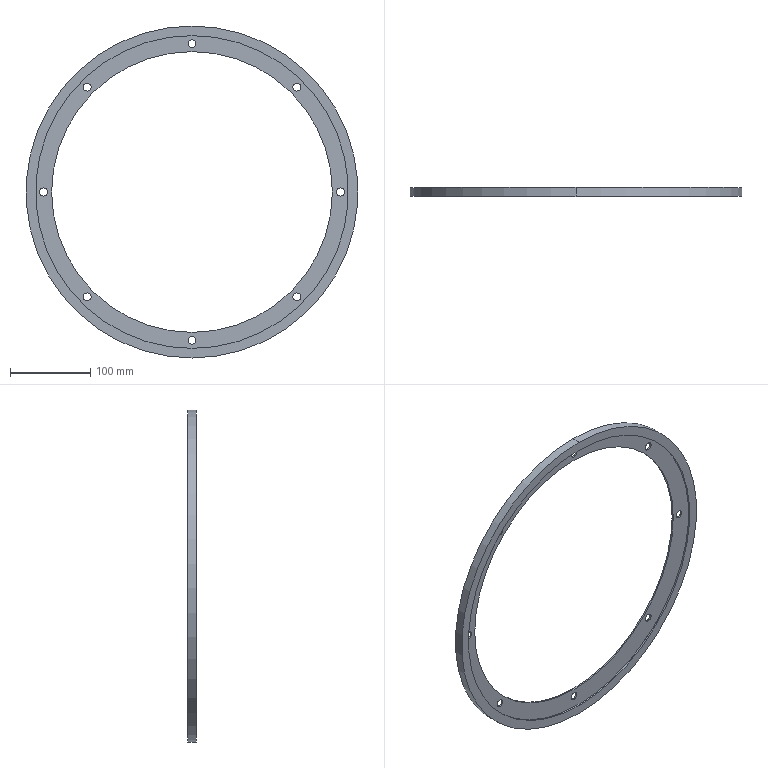Part | SolidWorks | features ICE 2, Extrusion 1 | 1 solid | 28 faces | box 414 x 11 x 414 mm | volume 123980 mm3 | cylinder 24 | plane 4 | commonest cylinder face diameters 10 x16 350 x2 390 x2 410 x2 414 x2
STEP:
#1=CARTESIAN_POINT('',(0.,-9.,195.));
#2=VERTEX_POINT('',#1);
#3=CARTESIAN_POINT('',(0.,-9.,-195.));
#4=VERTEX_POINT('',#3);
#5=CARTESIAN_POINT('',(0.,-9.,0.));
#6=DIRECTION('',(0.,-1.,0.));
#7=DIRECTION('',(0.,0.,-1.));
#8=AXIS2_PLACEMENT_3D('',#5,#6,#7);
#9=CIRCLE('',#8,195.);
#10=EDGE_CURVE('',#2,#4,#9,.T.);
#11=ORIENTED_EDGE('',*,*,#10,.T.);
#12=CARTESIAN_POINT('',(0.,-7.,-195.));
#13=VERTEX_POINT('',#12);
#14=CARTESIAN_POINT('',(0.,-9.,-195.));
#15=DIRECTION('',(0.,1.,0.));
#16=VECTOR('',#15,1000.);
#17=LINE('',#14,#16);
#18=EDGE_CURVE('',#4,#13,#17,.T.);
#19=ORIENTED_EDGE('',*,*,#18,.T.);
#20=CARTESIAN_POINT('',(0.,-7.,195.));
#21=VERTEX_POINT('',#20);
#22=CARTESIAN_POINT('',(0.,-7.,0.));
#23=DIRECTION('',(0.,-1.,0.));
#24=DIRECTION('',(0.,0.,-1.));
#25=AXIS2_PLACEMENT_3D('',#22,#23,#24);
#26=CIRCLE('',#25,195.);
#27=EDGE_CURVE('',#21,#13,#26,.T.);
#28=ORIENTED_EDGE('',*,*,#27,.F.);
#29=CARTESIAN_POINT('',(0.,-9.,195.));
#30=DIRECTION('',(0.,1.,0.));
#31=VECTOR('',#30,1000.);
#32=LINE('',#29,#31);
#33=EDGE_CURVE('',#2,#21,#32,.T.);
#34=ORIENTED_EDGE('',*,*,#33,.F.);
#35=EDGE_LOOP('',(#11,#19,#28,#34));
#36=FACE_OUTER_BOUND('',#35,.T.);
#37=CARTESIAN_POINT('',(0.,-9.,0.));
#38=DIRECTION('',(0.,1.,0.));
#39=DIRECTION('',(0.,0.,1.));
#40=AXIS2_PLACEMENT_3D('',#37,#38,#39);
#41=CYLINDRICAL_SURFACE('',#40,195.);
#42=ADVANCED_FACE('',(#36),#41,.F.);
#43=CARTESIAN_POINT('',(0.,2.,-207.));
#44=VERTEX_POINT('',#43);
#45=CARTESIAN_POINT('',(0.,2.,207.));
#46=VERTEX_POINT('',#45);
#47=CARTESIAN_POINT('',(0.,2.,0.));
#48=DIRECTION('',(0.,-1.,0.));
#49=DIRECTION('',(0.,0.,-1.));
#50=AXIS2_PLACEMENT_3D('',#47,#48,#49);
#51=CIRCLE('',#50,207.);
#52=EDGE_CURVE('',#44,#46,#51,.T.);
#53=ORIENTED_EDGE('',*,*,#52,.T.);
#54=CARTESIAN_POINT('',(0.,-9.,207.));
#55=VERTEX_POINT('',#54);
#56=CARTESIAN_POINT('',(0.,2.,207.));
#57=DIRECTION('',(0.,-1.,0.));
#58=VECTOR('',#57,1000.);
#59=LINE('',#56,#58);
#60=EDGE_CURVE('',#46,#55,#59,.T.);
#61=ORIENTED_EDGE('',*,*,#60,.T.);
#62=CARTESIAN_POINT('',(0.,-9.,-207.));
#63=VERTEX_POINT('',#62);
#64=CARTESIAN_POINT('',(0.,-9.,0.));
#65=DIRECTION('',(0.,-1.,0.));
#66=DIRECTION('',(0.,0.,-1.));
#67=AXIS2_PLACEMENT_3D('',#64,#65,#66);
#68=CIRCLE('',#67,207.);
#69=EDGE_CURVE('',#63,#55,#68,.T.);
#70=ORIENTED_EDGE('',*,*,#69,.F.);
#71=CARTESIAN_POINT('',(0.,2.,-207.));
#72=DIRECTION('',(0.,-1.,0.));
#73=VECTOR('',#72,1000.);
#74=LINE('',#71,#73);
#75=EDGE_CURVE('',#44,#63,#74,.T.);
#76=ORIENTED_EDGE('',*,*,#75,.F.);
#77=EDGE_LOOP('',(#53,#61,#70,#76));
#78=FACE_OUTER_BOUND('',#77,.T.);
#79=CARTESIAN_POINT('',(0.,2.,0.));
#80=DIRECTION('',(0.,-1.,0.));
#81=DIRECTION('',(0.,0.,-1.));
#82=AXIS2_PLACEMENT_3D('',#79,#80,#81);
#83=CYLINDRICAL_SURFACE('',#82,207.);
#84=ADVANCED_FACE('',(#78),#83,.T.);
#85=CARTESIAN_POINT('',(0.,0.,-205.));
#86=VERTEX_POINT('',#85);
#87=CARTESIAN_POINT('',(0.,0.,205.));
#88=VERTEX_POINT('',#87);
#89=CARTESIAN_POINT('',(0.,0.,0.));
#90=DIRECTION('',(0.,1.,0.));
#91=DIRECTION('',(0.,0.,1.));
#92=AXIS2_PLACEMENT_3D('',#89,#90,#91);
#93=CIRCLE('',#92,205.);
#94=EDGE_CURVE('',#86,#88,#93,.T.);
#95=ORIENTED_EDGE('',*,*,#94,.T.);
#96=CARTESIAN_POINT('',(0.,-7.,205.));
#97=VERTEX_POINT('',#96);
#98=CARTESIAN_POINT('',(0.,2.,205.));
#99=DIRECTION('',(0.,-1.,0.));
#100=VECTOR('',#99,1000.);
#101=LINE('',#98,#100);
#102=EDGE_CURVE('',#88,#97,#101,.T.);
#103=ORIENTED_EDGE('',*,*,#102,.T.);
#104=CARTESIAN_POINT('',(0.,-7.,-205.));
#105=VERTEX_POINT('',#104);
#106=CARTESIAN_POINT('',(0.,-7.,0.));
#107=DIRECTION('',(0.,-1.,0.));
#108=DIRECTION('',(0.,0.,-1.));
#109=AXIS2_PLACEMENT_3D('',#106,#107,#108);
#110=CIRCLE('',#109,205.);
#111=EDGE_CURVE('',#97,#105,#110,.T.);
#112=ORIENTED_EDGE('',*,*,#111,.T.);
#113=CARTESIAN_POINT('',(0.,2.,-205.));
#114=DIRECTION('',(0.,-1.,0.));
#115=VECTOR('',#114,1000.);
#116=LINE('',#113,#115);
#117=EDGE_CURVE('',#86,#105,#116,.T.);
#118=ORIENTED_EDGE('',*,*,#117,.F.);
#119=EDGE_LOOP('',(#95,#103,#112,#118));
#120=FACE_OUTER_BOUND('',#119,.T.);
#121=CARTESIAN_POINT('',(0.,2.,0.));
#122=DIRECTION('',(0.,-1.,0.));
#123=DIRECTION('',(0.,0.,-1.));
#124=AXIS2_PLACEMENT_3D('',#121,#122,#123);
#125=CYLINDRICAL_SURFACE('',#124,205.);
#126=ADVANCED_FACE('',(#120),#125,.F.);
#127=CARTESIAN_POINT('',(-130.815,2.,125.815));
#128=VERTEX_POINT('',#127);
#129=CARTESIAN_POINT('',(-130.815,2.,135.815));
#130=VERTEX_POINT('',#129);
#131=CARTESIAN_POINT('',(-130.815,2.,130.815));
#132=DIRECTION('',(0.,1.,0.));
#133=DIRECTION('',(0.,0.,1.));
#134=AXIS2_PLACEMENT_3D('',#131,#132,#133);
#135=CIRCLE('',#134,5.);
#136=EDGE_CURVE('',#128,#130,#135,.T.);
#137=ORIENTED_EDGE('',*,*,#136,.T.);
#138=CARTESIAN_POINT('',(-130.815,0.,135.815));
#139=VERTEX_POINT('',#138);
#140=CARTESIAN_POINT('',(-130.815,2.,135.815));
#141=DIRECTION('',(0.,-1.,0.));
#142=VECTOR('',#141,1000.);
#143=LINE('',#140,#142);
#144=EDGE_CURVE('',#130,#139,#143,.T.);
#145=ORIENTED_EDGE('',*,*,#144,.T.);
#146=CARTESIAN_POINT('',(-130.815,0.,125.815));
#147=VERTEX_POINT('',#146);
#148=CARTESIAN_POINT('',(-130.815,0.,130.815));
#149=DIRECTION('',(0.,1.,0.));
#150=DIRECTION('',(0.,0.,1.));
#151=AXIS2_PLACEMENT_3D('',#148,#149,#150);
#152=CIRCLE('',#151,5.);
#153=EDGE_CURVE('',#147,#139,#152,.T.);
#154=ORIENTED_EDGE('',*,*,#153,.F.);
#155=CARTESIAN_POINT('',(-130.815,2.,125.815));
#156=DIRECTION('',(0.,-1.,0.));
#157=VECTOR('',#156,1000.);
#158=LINE('',#155,#157);
#159=EDGE_CURVE('',#128,#147,#158,.T.);
#160=ORIENTED_EDGE('',*,*,#159,.F.);
#161=EDGE_LOOP('',(#137,#145,#154,#160));
#162=FACE_OUTER_BOUND('',#161,.T.);
#163=CARTESIAN_POINT('',(-130.815,2.,130.815));
#164=DIRECTION('',(0.,-1.,0.));
#165=DIRECTION('',(0.,0.,-1.));
#166=AXIS2_PLACEMENT_3D('',#163,#164,#165);
#167=CYLINDRICAL_SURFACE('',#166,5.);
#168=ADVANCED_FACE('',(#162),#167,.F.);
#169=CARTESIAN_POINT('',(0.,2.,180.));
#170=VERTEX_POINT('',#169);
#171=CARTESIAN_POINT('',(0.,2.,190.));
#172=VERTEX_POINT('',#171);
#173=CARTESIAN_POINT('',(0.,2.,185.));
#174=DIRECTION('',(0.,1.,0.));
#175=DIRECTION('',(0.,0.,1.));
#176=AXIS2_PLACEMENT_3D('',#173,#174,#175);
#177=CIRCLE('',#176,5.);
#178=EDGE_CURVE('',#170,#172,#177,.T.);
#179=ORIENTED_EDGE('',*,*,#178,.T.);
#180=CARTESIAN_POINT('',(0.,0.,190.));
#181=VERTEX_POINT('',#180);
#182=CARTESIAN_POINT('',(0.,2.,190.));
#183=DIRECTION('',(0.,-1.,0.));
#184=VECTOR('',#183,1000.);
#185=LINE('',#182,#184);
#186=EDGE_CURVE('',#172,#181,#185,.T.);
#187=ORIENTED_EDGE('',*,*,#186,.T.);
#188=CARTESIAN_POINT('',(0.,0.,180.));
#189=VERTEX_POINT('',#188);
#190=CARTESIAN_POINT('',(0.,0.,185.));
#191=DIRECTION('',(0.,1.,0.));
#192=DIRECTION('',(0.,0.,1.));
#193=AXIS2_PLACEMENT_3D('',#190,#191,#192);
#194=CIRCLE('',#193,5.);
#195=EDGE_CURVE('',#189,#181,#194,.T.);
#196=ORIENTED_EDGE('',*,*,#195,.F.);
#197=CARTESIAN_POINT('',(0.,2.,180.));
#198=DIRECTION('',(0.,-1.,0.));
#199=VECTOR('',#198,1000.);
#200=LINE('',#197,#199);
#201=EDGE_CURVE('',#170,#189,#200,.T.);
#202=ORIENTED_EDGE('',*,*,#201,.F.);
#203=EDGE_LOOP('',(#179,#187,#196,#202));
#204=FACE_OUTER_BOUND('',#203,.T.);
#205=CARTESIAN_POINT('',(0.,2.,185.));
#206=DIRECTION('',(0.,-1.,0.));
#207=DIRECTION('',(0.,0.,-1.));
#208=AXIS2_PLACEMENT_3D('',#205,#206,#207);
#209=CYLINDRICAL_SURFACE('',#208,5.);
#210=ADVANCED_FACE('',(#204),#209,.F.);
#211=CARTESIAN_POINT('',(130.815,2.,125.815));
#212=VERTEX_POINT('',#211);
#213=CARTESIAN_POINT('',(130.815,2.,135.815));
#214=VERTEX_POINT('',#213);
#215=CARTESIAN_POINT('',(130.815,2.,130.815));
#216=DIRECTION('',(0.,1.,0.));
#217=DIRECTION('',(0.,0.,1.));
#218=AXIS2_PLACEMENT_3D('',#215,#216,#217);
#219=CIRCLE('',#218,5.);
#220=EDGE_CURVE('',#212,#214,#219,.T.);
#221=ORIENTED_EDGE('',*,*,#220,.T.);
#222=CARTESIAN_POINT('',(130.815,0.,135.815));
#223=VERTEX_POINT('',#222);
#224=CARTESIAN_POINT('',(130.815,2.,135.815));
#225=DIRECTION('',(0.,-1.,0.));
#226=VECTOR('',#225,1000.);
#227=LINE('',#224,#226);
#228=EDGE_CURVE('',#214,#223,#227,.T.);
#229=ORIENTED_EDGE('',*,*,#228,.T.);
#230=CARTESIAN_POINT('',(130.815,0.,125.815));
#231=VERTEX_POINT('',#230);
#232=CARTESIAN_POINT('',(130.815,0.,130.815));
#233=DIRECTION('',(0.,1.,0.));
#234=DIRECTION('',(0.,0.,1.));
#235=AXIS2_PLACEMENT_3D('',#232,#233,#234);
#236=CIRCLE('',#235,5.);
#237=EDGE_CURVE('',#231,#223,#236,.T.);
#238=ORIENTED_EDGE('',*,*,#237,.F.);
#239=CARTESIAN_POINT('',(130.815,2.,125.815));
#240=DIRECTION('',(0.,-1.,0.));
#241=VECTOR('',#240,1000.);
#242=LINE('',#239,#241);
#243=EDGE_CURVE('',#212,#231,#242,.T.);
#244=ORIENTED_EDGE('',*,*,#243,.F.);
#245=EDGE_LOOP('',(#221,#229,#238,#244));
#246=FACE_OUTER_BOUND('',#245,.T.);
#247=CARTESIAN_POINT('',(130.815,2.,130.815));
#248=DIRECTION('',(0.,-1.,0.));
#249=DIRECTION('',(0.,0.,-1.));
#250=AXIS2_PLACEMENT_3D('',#247,#248,#249);
#251=CYLINDRICAL_SURFACE('',#250,5.);
#252=ADVANCED_FACE('',(#246),#251,.F.);
#253=CARTESIAN_POINT('',(185.,2.,-5.));
#254=VERTEX_POINT('',#253);
#255=CARTESIAN_POINT('',(185.,2.,5.));
#256=VERTEX_POINT('',#255);
#257=CARTESIAN_POINT('',(185.,2.,0.));
#258=DIRECTION('',(0.,1.,0.));
#259=DIRECTION('',(0.,0.,1.));
#260=AXIS2_PLACEMENT_3D('',#257,#258,#259);
#261=CIRCLE('',#260,5.);
#262=EDGE_CURVE('',#254,#256,#261,.T.);
#263=ORIENTED_EDGE('',*,*,#262,.T.);
#264=CARTESIAN_POINT('',(185.,0.,5.));
#265=VERTEX_POINT('',#264);
#266=CARTESIAN_POINT('',(185.,2.,5.));
#267=DIRECTION('',(0.,-1.,0.));
#268=VECTOR('',#267,1000.);
#269=LINE('',#266,#268);
#270=EDGE_CURVE('',#256,#265,#269,.T.);
#271=ORIENTED_EDGE('',*,*,#270,.T.);
#272=CARTESIAN_POINT('',(185.,0.,-5.));
#273=VERTEX_POINT('',#272);
#274=CARTESIAN_POINT('',(185.,0.,0.));
#275=DIRECTION('',(0.,1.,0.));
#276=DIRECTION('',(0.,0.,1.));
#277=AXIS2_PLACEMENT_3D('',#274,#275,#276);
#278=CIRCLE('',#277,5.);
#279=EDGE_CURVE('',#273,#265,#278,.T.);
#280=ORIENTED_EDGE('',*,*,#279,.F.);
#281=CARTESIAN_POINT('',(185.,2.,-5.));
#282=DIRECTION('',(0.,-1.,0.));
#283=VECTOR('',#282,1000.);
#284=LINE('',#281,#283);
#285=EDGE_CURVE('',#254,#273,#284,.T.);
#286=ORIENTED_EDGE('',*,*,#285,.F.);
#287=EDGE_LOOP('',(#263,#271,#280,#286));
#288=FACE_OUTER_BOUND('',#287,.T.);
#289=CARTESIAN_POINT('',(185.,2.,0.));
#290=DIRECTION('',(0.,-1.,0.));
#291=DIRECTION('',(0.,0.,-1.));
#292=AXIS2_PLACEMENT_3D('',#289,#290,#291);
#293=CYLINDRICAL_SURFACE('',#292,5.);
#294=ADVANCED_FACE('',(#288),#293,.F.);
#295=CARTESIAN_POINT('',(130.815,2.,-135.815));
#296=VERTEX_POINT('',#295);
#297=CARTESIAN_POINT('',(130.815,2.,-125.815));
#298=VERTEX_POINT('',#297);
#299=CARTESIAN_POINT('',(130.815,2.,-130.815));
#300=DIRECTION('',(0.,1.,0.));
#301=DIRECTION('',(0.,0.,1.));
#302=AXIS2_PLACEMENT_3D('',#299,#300,#301);
#303=CIRCLE('',#302,5.);
#304=EDGE_CURVE('',#296,#298,#303,.T.);
#305=ORIENTED_EDGE('',*,*,#304,.T.);
#306=CARTESIAN_POINT('',(130.815,0.,-125.815));
#307=VERTEX_POINT('',#306);
#308=CARTESIAN_POINT('',(130.815,2.,-125.815));
#309=DIRECTION('',(0.,-1.,0.));
#310=VECTOR('',#309,1000.);
#311=LINE('',#308,#310);
#312=EDGE_CURVE('',#298,#307,#311,.T.);
#313=ORIENTED_EDGE('',*,*,#312,.T.);
#314=CARTESIAN_POINT('',(130.815,0.,-135.815));
#315=VERTEX_POINT('',#314);
#316=CARTESIAN_POINT('',(130.815,0.,-130.815));
#317=DIRECTION('',(0.,1.,0.));
#318=DIRECTION('',(0.,0.,1.));
#319=AXIS2_PLACEMENT_3D('',#316,#317,#318);
#320=CIRCLE('',#319,5.);
#321=EDGE_CURVE('',#315,#307,#320,.T.);
#322=ORIENTED_EDGE('',*,*,#321,.F.);
#323=CARTESIAN_POINT('',(130.815,2.,-135.815));
#324=DIRECTION('',(0.,-1.,0.));
#325=VECTOR('',#324,1000.);
#326=LINE('',#323,#325);
#327=EDGE_CURVE('',#296,#315,#326,.T.);
#328=ORIENTED_EDGE('',*,*,#327,.F.);
#329=EDGE_LOOP('',(#305,#313,#322,#328));
#330=FACE_OUTER_BOUND('',#329,.T.);
#331=CARTESIAN_POINT('',(130.815,2.,-130.815));
#332=DIRECTION('',(0.,-1.,0.));
#333=DIRECTION('',(0.,0.,-1.));
#334=AXIS2_PLACEMENT_3D('',#331,#332,#333);
#335=CYLINDRICAL_SURFACE('',#334,5.);
#336=ADVANCED_FACE('',(#330),#335,.F.);
#337=CARTESIAN_POINT('',(0.,2.,-190.));
#338=VERTEX_POINT('',#337);
#339=CARTESIAN_POINT('',(0.,2.,-180.));
#340=VERTEX_POINT('',#339);
#341=CARTESIAN_POINT('',(0.,2.,-185.));
#342=DIRECTION('',(0.,1.,0.));
#343=DIRECTION('',(0.,0.,1.));
#344=AXIS2_PLACEMENT_3D('',#341,#342,#343);
#345=CIRCLE('',#344,5.);
#346=EDGE_CURVE('',#338,#340,#345,.T.);
#347=ORIENTED_EDGE('',*,*,#346,.T.);
#348=CARTESIAN_POINT('',(0.,0.,-180.));
#349=VERTEX_POINT('',#348);
#350=CARTESIAN_POINT('',(0.,2.,-180.));
#351=DIRECTION('',(0.,-1.,0.));
#352=VECTOR('',#351,1000.);
#353=LINE('',#350,#352);
#354=EDGE_CURVE('',#340,#349,#353,.T.);
#355=ORIENTED_EDGE('',*,*,#354,.T.);
#356=CARTESIAN_POINT('',(0.,0.,-190.));
#357=VERTEX_POINT('',#356);
#358=CARTESIAN_POINT('',(0.,0.,-185.));
#359=DIRECTION('',(0.,1.,0.));
#360=DIRECTION('',(0.,0.,1.));
#361=AXIS2_PLACEMENT_3D('',#358,#359,#360);
#362=CIRCLE('',#361,5.);
#363=EDGE_CURVE('',#357,#349,#362,.T.);
#364=ORIENTED_EDGE('',*,*,#363,.F.);
#365=CARTESIAN_POINT('',(0.,2.,-190.));
#366=DIRECTION('',(0.,-1.,0.));
#367=VECTOR('',#366,1000.);
#368=LINE('',#365,#367);
#369=EDGE_CURVE('',#338,#357,#368,.T.);
#370=ORIENTED_EDGE('',*,*,#369,.F.);
#371=EDGE_LOOP('',(#347,#355,#364,#370));
#372=FACE_OUTER_BOUND('',#371,.T.);
#373=CARTESIAN_POINT('',(0.,2.,-185.));
#374=DIRECTION('',(0.,-1.,0.));
#375=DIRECTION('',(0.,0.,-1.));
#376=AXIS2_PLACEMENT_3D('',#373,#374,#375);
#377=CYLINDRICAL_SURFACE('',#376,5.);
#378=ADVANCED_FACE('',(#372),#377,.F.);
#379=CARTESIAN_POINT('',(-130.815,2.,-135.815));
#380=VERTEX_POINT('',#379);
#381=CARTESIAN_POINT('',(-130.815,2.,-125.815));
#382=VERTEX_POINT('',#381);
#383=CARTESIAN_POINT('',(-130.815,2.,-130.815));
#384=DIRECTION('',(0.,1.,0.));
#385=DIRECTION('',(0.,0.,1.));
#386=AXIS2_PLACEMENT_3D('',#383,#384,#385);
#387=CIRCLE('',#386,5.);
#388=EDGE_CURVE('',#380,#382,#387,.T.);
#389=ORIENTED_EDGE('',*,*,#388,.T.);
#390=CARTESIAN_POINT('',(-130.815,0.,-125.815));
#391=VERTEX_POINT('',#390);
#392=CARTESIAN_POINT('',(-130.815,2.,-125.815));
#393=DIRECTION('',(0.,-1.,0.));
#394=VECTOR('',#393,1000.);
#395=LINE('',#392,#394);
#396=EDGE_CURVE('',#382,#391,#395,.T.);
#397=ORIENTED_EDGE('',*,*,#396,.T.);
#398=CARTESIAN_POINT('',(-130.815,0.,-135.815));
#399=VERTEX_POINT('',#398);
#400=CARTESIAN_POINT('',(-130.815,0.,-130.815));
#401=DIRECTION('',(0.,1.,0.));
#402=DIRECTION('',(0.,0.,1.));
#403=AXIS2_PLACEMENT_3D('',#400,#401,#402);
#404=CIRCLE('',#403,5.);
#405=EDGE_CURVE('',#399,#391,#404,.T.);
#406=ORIENTED_EDGE('',*,*,#405,.F.);
#407=CARTESIAN_POINT('',(-130.815,2.,-135.815));
#408=DIRECTION('',(0.,-1.,0.));
#409=VECTOR('',#408,1000.);
#410=LINE('',#407,#409);
#411=EDGE_CURVE('',#380,#399,#410,.T.);
#412=ORIENTED_EDGE('',*,*,#411,.F.);
#413=EDGE_LOOP('',(#389,#397,#406,#412));
#414=FACE_OUTER_BOUND('',#413,.T.);
#415=CARTESIAN_POINT('',(-130.815,2.,-130.815));
#416=DIRECTION('',(0.,-1.,0.));
#417=DIRECTION('',(0.,0.,-1.));
#418=AXIS2_PLACEMENT_3D('',#415,#416,#417);
#419=CYLINDRICAL_SURFACE('',#418,5.);
#420=ADVANCED_FACE('',(#414),#419,.F.);
#421=CARTESIAN_POINT('',(0.,2.,-175.));
#422=VERTEX_POINT('',#421);
#423=CARTESIAN_POINT('',(0.,2.,175.));
#424=VERTEX_POINT('',#423);
#425=CARTESIAN_POINT('',(0.,2.,0.));
#426=DIRECTION('',(0.,1.,0.));
#427=DIRECTION('',(0.,0.,1.));
#428=AXIS2_PLACEMENT_3D('',#425,#426,#427);
#429=CIRCLE('',#428,175.);
#430=EDGE_CURVE('',#422,#424,#429,.T.);
#431=ORIENTED_EDGE('',*,*,#430,.T.);
#432=CARTESIAN_POINT('',(0.,0.,175.));
#433=VERTEX_POINT('',#432);
#434=CARTESIAN_POINT('',(0.,2.,175.));
#435=DIRECTION('',(0.,-1.,0.));
#436=VECTOR('',#435,1000.);
#437=LINE('',#434,#436);
#438=EDGE_CURVE('',#424,#433,#437,.T.);
#439=ORIENTED_EDGE('',*,*,#438,.T.);
#440=CARTESIAN_POINT('',(0.,0.,-175.));
#441=VERTEX_POINT('',#440);
#442=CARTESIAN_POINT('',(0.,0.,0.));
#443=DIRECTION('',(0.,1.,0.));
#444=DIRECTION('',(0.,0.,1.));
#445=AXIS2_PLACEMENT_3D('',#442,#443,#444);
#446=CIRCLE('',#445,175.);
#447=EDGE_CURVE('',#441,#433,#446,.T.);
#448=ORIENTED_EDGE('',*,*,#447,.F.);
#449=CARTESIAN_POINT('',(0.,2.,-175.));
#450=DIRECTION('',(0.,-1.,0.));
#451=VECTOR('',#450,1000.);
#452=LINE('',#449,#451);
#453=EDGE_CURVE('',#422,#441,#452,.T.);
#454=ORIENTED_EDGE('',*,*,#453,.F.);
#455=EDGE_LOOP('',(#431,#439,#448,#454));
#456=FACE_OUTER_BOUND('',#455,.T.);
#457=CARTESIAN_POINT('',(0.,2.,0.));
#458=DIRECTION('',(0.,-1.,0.));
#459=DIRECTION('',(0.,0.,-1.));
#460=AXIS2_PLACEMENT_3D('',#457,#458,#459);
#461=CYLINDRICAL_SURFACE('',#460,175.);
#462=ADVANCED_FACE('',(#456),#461,.F.);
#463=CARTESIAN_POINT('',(-185.,2.,-5.));
#464=VERTEX_POINT('',#463);
#465=CARTESIAN_POINT('',(-185.,2.,5.));
#466=VERTEX_POINT('',#465);
#467=CARTESIAN_POINT('',(-185.,2.,0.));
#468=DIRECTION('',(0.,1.,0.));
#469=DIRECTION('',(0.,0.,1.));
#470=AXIS2_PLACEMENT_3D('',#467,#468,#469);
#471=CIRCLE('',#470,5.);
#472=EDGE_CURVE('',#464,#466,#471,.T.);
#473=ORIENTED_EDGE('',*,*,#472,.T.);
#474=CARTESIAN_POINT('',(-185.,0.,5.));
#475=VERTEX_POINT('',#474);
#476=CARTESIAN_POINT('',(-185.,2.,5.));
#477=DIRECTION('',(0.,-1.,0.));
#478=VECTOR('',#477,1000.);
#479=LINE('',#476,#478);
#480=EDGE_CURVE('',#466,#475,#479,.T.);
#481=ORIENTED_EDGE('',*,*,#480,.T.);
#482=CARTESIAN_POINT('',(-185.,0.,-5.));
#483=VERTEX_POINT('',#482);
#484=CARTESIAN_POINT('',(-185.,0.,0.));
#485=DIRECTION('',(0.,1.,0.));
#486=DIRECTION('',(0.,0.,1.));
#487=AXIS2_PLACEMENT_3D('',#484,#485,#486);
#488=CIRCLE('',#487,5.);
#489=EDGE_CURVE('',#483,#475,#488,.T.);
#490=ORIENTED_EDGE('',*,*,#489,.F.);
#491=CARTESIAN_POINT('',(-185.,2.,-5.));
#492=DIRECTION('',(0.,-1.,0.));
#493=VECTOR('',#492,1000.);
#494=LINE('',#491,#493);
#495=EDGE_CURVE('',#464,#483,#494,.T.);
#496=ORIENTED_EDGE('',*,*,#495,.F.);
#497=EDGE_LOOP('',(#473,#481,#490,#496));
#498=FACE_OUTER_BOUND('',#497,.T.);
#499=CARTESIAN_POINT('',(-185.,2.,0.));
#500=DIRECTION('',(0.,-1.,0.));
#501=DIRECTION('',(0.,0.,-1.));
#502=AXIS2_PLACEMENT_3D('',#499,#500,#501);
#503=CYLINDRICAL_SURFACE('',#502,5.);
#504=ADVANCED_FACE('',(#498),#503,.F.);
#505=ORIENTED_EDGE('',*,*,#178,.F.);
#506=CARTESIAN_POINT('',(0.,2.,185.));
#507=DIRECTION('',(0.,1.,0.));
#508=DIRECTION('',(0.,0.,1.));
#509=AXIS2_PLACEMENT_3D('',#506,#507,#508);
#510=CIRCLE('',#509,5.);
#511=EDGE_CURVE('',#172,#170,#510,.T.);
#512=ORIENTED_EDGE('',*,*,#511,.F.);
#513=EDGE_LOOP('',(#505,#512));
#514=FACE_BOUND('',#513,.T.);
#515=ORIENTED_EDGE('',*,*,#262,.F.);
#516=CARTESIAN_POINT('',(185.,2.,0.));
#517=DIRECTION('',(0.,1.,0.));
#518=DIRECTION('',(0.,0.,1.));
#519=AXIS2_PLACEMENT_3D('',#516,#517,#518);
#520=CIRCLE('',#519,5.);
#521=EDGE_CURVE('',#256,#254,#520,.T.);
#522=ORIENTED_EDGE('',*,*,#521,.F.);
#523=EDGE_LOOP('',(#515,#522));
#524=FACE_BOUND('',#523,.T.);
#525=ORIENTED_EDGE('',*,*,#346,.F.);
#526=CARTESIAN_POINT('',(0.,2.,-185.));
#527=DIRECTION('',(0.,1.,0.));
#528=DIRECTION('',(0.,0.,1.));
#529=AXIS2_PLACEMENT_3D('',#526,#527,#528);
#530=CIRCLE('',#529,5.);
#531=EDGE_CURVE('',#340,#338,#530,.T.);
#532=ORIENTED_EDGE('',*,*,#531,.F.);
#533=EDGE_LOOP('',(#525,#532));
#534=FACE_BOUND('',#533,.T.);
#535=ORIENTED_EDGE('',*,*,#430,.F.);
#536=CARTESIAN_POINT('',(0.,2.,0.));
#537=DIRECTION('',(0.,1.,0.));
#538=DIRECTION('',(0.,0.,1.));
#539=AXIS2_PLACEMENT_3D('',#536,#537,#538);
#540=CIRCLE('',#539,175.);
#541=EDGE_CURVE('',#424,#422,#540,.T.);
#542=ORIENTED_EDGE('',*,*,#541,.F.);
#543=EDGE_LOOP('',(#535,#542));
#544=FACE_BOUND('',#543,.T.);
#545=ORIENTED_EDGE('',*,*,#472,.F.);
#546=CARTESIAN_POINT('',(-185.,2.,0.));
#547=DIRECTION('',(0.,1.,0.));
#548=DIRECTION('',(0.,0.,1.));
#549=AXIS2_PLACEMENT_3D('',#546,#547,#548);
#550=CIRCLE('',#549,5.);
#551=EDGE_CURVE('',#466,#464,#550,.T.);
#552=ORIENTED_EDGE('',*,*,#551,.F.);
#553=EDGE_LOOP('',(#545,#552));
#554=FACE_BOUND('',#553,.T.);
#555=ORIENTED_EDGE('',*,*,#388,.F.);
#556=CARTESIAN_POINT('',(-130.815,2.,-130.815));
#557=DIRECTION('',(0.,1.,0.));
#558=DIRECTION('',(0.,0.,1.));
#559=AXIS2_PLACEMENT_3D('',#556,#557,#558);
#560=CIRCLE('',#559,5.);
#561=EDGE_CURVE('',#382,#380,#560,.T.);
#562=ORIENTED_EDGE('',*,*,#561,.F.);
#563=EDGE_LOOP('',(#555,#562));
#564=FACE_BOUND('',#563,.T.);
#565=ORIENTED_EDGE('',*,*,#304,.F.);
#566=CARTESIAN_POINT('',(130.815,2.,-130.815));
#567=DIRECTION('',(0.,1.,0.));
#568=DIRECTION('',(0.,0.,1.));
#569=AXIS2_PLACEMENT_3D('',#566,#567,#568);
#570=CIRCLE('',#569,5.);
#571=EDGE_CURVE('',#298,#296,#570,.T.);
#572=ORIENTED_EDGE('',*,*,#571,.F.);
#573=EDGE_LOOP('',(#565,#572));
#574=FACE_BOUND('',#573,.T.);
#575=ORIENTED_EDGE('',*,*,#220,.F.);
#576=CARTESIAN_POINT('',(130.815,2.,130.815));
#577=DIRECTION('',(0.,1.,0.));
#578=DIRECTION('',(0.,0.,1.));
#579=AXIS2_PLACEMENT_3D('',#576,#577,#578);
#580=CIRCLE('',#579,5.);
#581=EDGE_CURVE('',#214,#212,#580,.T.);
#582=ORIENTED_EDGE('',*,*,#581,.F.);
#583=EDGE_LOOP('',(#575,#582));
#584=FACE_BOUND('',#583,.T.);
#585=ORIENTED_EDGE('',*,*,#136,.F.);
#586=CARTESIAN_POINT('',(-130.815,2.,130.815));
#587=DIRECTION('',(0.,1.,0.));
#588=DIRECTION('',(0.,0.,1.));
#589=AXIS2_PLACEMENT_3D('',#586,#587,#588);
#590=CIRCLE('',#589,5.);
#591=EDGE_CURVE('',#130,#128,#590,.T.);
#592=ORIENTED_EDGE('',*,*,#591,.F.);
#593=EDGE_LOOP('',(#585,#592));
#594=FACE_BOUND('',#593,.T.);
#595=ORIENTED_EDGE('',*,*,#52,.F.);
#596=CARTESIAN_POINT('',(0.,2.,0.));
#597=DIRECTION('',(0.,-1.,0.));
#598=DIRECTION('',(0.,0.,-1.));
#599=AXIS2_PLACEMENT_3D('',#596,#597,#598);
#600=CIRCLE('',#599,207.);
#601=EDGE_CURVE('',#46,#44,#600,.T.);
#602=ORIENTED_EDGE('',*,*,#601,.F.);
#603=EDGE_LOOP('',(#595,#602));
#604=FACE_OUTER_BOUND('',#603,.T.);
#605=CARTESIAN_POINT('',(0.,2.,0.));
#606=DIRECTION('',(0.,1.,0.));
#607=DIRECTION('',(0.,0.,1.));
#608=AXIS2_PLACEMENT_3D('',#605,#606,#607);
#609=PLANE('',#608);
#610=ADVANCED_FACE('',(#514,#524,#534,#544,#554,#564,#574,#584,#594,#604),#609,.T.);
#611=ORIENTED_EDGE('',*,*,#94,.F.);
#612=CARTESIAN_POINT('',(0.,0.,0.));
#613=DIRECTION('',(0.,1.,0.));
#614=DIRECTION('',(0.,0.,1.));
#615=AXIS2_PLACEMENT_3D('',#612,#613,#614);
#616=CIRCLE('',#615,205.);
#617=EDGE_CURVE('',#88,#86,#616,.T.);
#618=ORIENTED_EDGE('',*,*,#617,.F.);
#619=EDGE_LOOP('',(#611,#618));
#620=FACE_OUTER_BOUND('',#619,.T.);
#621=ORIENTED_EDGE('',*,*,#489,.T.);
#622=CARTESIAN_POINT('',(-185.,0.,0.));
#623=DIRECTION('',(0.,1.,0.));
#624=DIRECTION('',(0.,0.,1.));
#625=AXIS2_PLACEMENT_3D('',#622,#623,#624);
#626=CIRCLE('',#625,5.);
#627=EDGE_CURVE('',#475,#483,#626,.T.);
#628=ORIENTED_EDGE('',*,*,#627,.T.);
#629=EDGE_LOOP('',(#621,#628));
#630=FACE_BOUND('',#629,.T.);
#631=ORIENTED_EDGE('',*,*,#447,.T.);
#632=CARTESIAN_POINT('',(0.,0.,0.));
#633=DIRECTION('',(0.,1.,0.));
#634=DIRECTION('',(0.,0.,1.));
#635=AXIS2_PLACEMENT_3D('',#632,#633,#634);
#636=CIRCLE('',#635,175.);
#637=EDGE_CURVE('',#433,#441,#636,.T.);
#638=ORIENTED_EDGE('',*,*,#637,.T.);
#639=EDGE_LOOP('',(#631,#638));
#640=FACE_BOUND('',#639,.T.);
#641=ORIENTED_EDGE('',*,*,#405,.T.);
#642=CARTESIAN_POINT('',(-130.815,0.,-130.815));
#643=DIRECTION('',(0.,1.,0.));
#644=DIRECTION('',(0.,0.,1.));
#645=AXIS2_PLACEMENT_3D('',#642,#643,#644);
#646=CIRCLE('',#645,5.);
#647=EDGE_CURVE('',#391,#399,#646,.T.);
#648=ORIENTED_EDGE('',*,*,#647,.T.);
#649=EDGE_LOOP('',(#641,#648));
#650=FACE_BOUND('',#649,.T.);
#651=ORIENTED_EDGE('',*,*,#363,.T.);
#652=CARTESIAN_POINT('',(0.,0.,-185.));
#653=DIRECTION('',(0.,1.,0.));
#654=DIRECTION('',(0.,0.,1.));
#655=AXIS2_PLACEMENT_3D('',#652,#653,#654);
#656=CIRCLE('',#655,5.);
#657=EDGE_CURVE('',#349,#357,#656,.T.);
#658=ORIENTED_EDGE('',*,*,#657,.T.);
#659=EDGE_LOOP('',(#651,#658));
#660=FACE_BOUND('',#659,.T.);
#661=ORIENTED_EDGE('',*,*,#321,.T.);
#662=CARTESIAN_POINT('',(130.815,0.,-130.815));
#663=DIRECTION('',(0.,1.,0.));
#664=DIRECTION('',(0.,0.,1.));
#665=AXIS2_PLACEMENT_3D('',#662,#663,#664);
#666=CIRCLE('',#665,5.);
#667=EDGE_CURVE('',#307,#315,#666,.T.);
#668=ORIENTED_EDGE('',*,*,#667,.T.);
#669=EDGE_LOOP('',(#661,#668));
#670=FACE_BOUND('',#669,.T.);
#671=ORIENTED_EDGE('',*,*,#279,.T.);
#672=CARTESIAN_POINT('',(185.,0.,0.));
#673=DIRECTION('',(0.,1.,0.));
#674=DIRECTION('',(0.,0.,1.));
#675=AXIS2_PLACEMENT_3D('',#672,#673,#674);
#676=CIRCLE('',#675,5.);
#677=EDGE_CURVE('',#265,#273,#676,.T.);
#678=ORIENTED_EDGE('',*,*,#677,.T.);
#679=EDGE_LOOP('',(#671,#678));
#680=FACE_BOUND('',#679,.T.);
#681=ORIENTED_EDGE('',*,*,#237,.T.);
#682=CARTESIAN_POINT('',(130.815,0.,130.815));
#683=DIRECTION('',(0.,1.,0.));
#684=DIRECTION('',(0.,0.,1.));
#685=AXIS2_PLACEMENT_3D('',#682,#683,#684);
#686=CIRCLE('',#685,5.);
#687=EDGE_CURVE('',#223,#231,#686,.T.);
#688=ORIENTED_EDGE('',*,*,#687,.T.);
#689=EDGE_LOOP('',(#681,#688));
#690=FACE_BOUND('',#689,.T.);
#691=ORIENTED_EDGE('',*,*,#195,.T.);
#692=CARTESIAN_POINT('',(0.,0.,185.));
#693=DIRECTION('',(0.,1.,0.));
#694=DIRECTION('',(0.,0.,1.));
#695=AXIS2_PLACEMENT_3D('',#692,#693,#694);
#696=CIRCLE('',#695,5.);
#697=EDGE_CURVE('',#181,#189,#696,.T.);
#698=ORIENTED_EDGE('',*,*,#697,.T.);
#699=EDGE_LOOP('',(#691,#698));
#700=FACE_BOUND('',#699,.T.);
#701=ORIENTED_EDGE('',*,*,#153,.T.);
#702=CARTESIAN_POINT('',(-130.815,0.,130.815));
#703=DIRECTION('',(0.,1.,0.));
#704=DIRECTION('',(0.,0.,1.));
#705=AXIS2_PLACEMENT_3D('',#702,#703,#704);
#706=CIRCLE('',#705,5.);
#707=EDGE_CURVE('',#139,#147,#706,.T.);
#708=ORIENTED_EDGE('',*,*,#707,.T.);
#709=EDGE_LOOP('',(#701,#708));
#710=FACE_BOUND('',#709,.T.);
#711=CARTESIAN_POINT('',(0.,0.,0.));
#712=DIRECTION('',(0.,1.,0.));
#713=DIRECTION('',(0.,0.,1.));
#714=AXIS2_PLACEMENT_3D('',#711,#712,#713);
#715=PLANE('',#714);
#716=ADVANCED_FACE('',(#620,#630,#640,#650,#660,#670,#680,#690,#700,#710),#715,.F.);
#717=ORIENTED_EDGE('',*,*,#480,.F.);
#718=ORIENTED_EDGE('',*,*,#551,.T.);
#719=ORIENTED_EDGE('',*,*,#495,.T.);
#720=ORIENTED_EDGE('',*,*,#627,.F.);
#721=EDGE_LOOP('',(#717,#718,#719,#720));
#722=FACE_OUTER_BOUND('',#721,.T.);
#723=CARTESIAN_POINT('',(-185.,2.,0.));
#724=DIRECTION('',(0.,-1.,0.));
#725=DIRECTION('',(0.,0.,-1.));
#726=AXIS2_PLACEMENT_3D('',#723,#724,#725);
#727=CYLINDRICAL_SURFACE('',#726,5.);
#728=ADVANCED_FACE('',(#722),#727,.F.);
#729=ORIENTED_EDGE('',*,*,#438,.F.);
#730=ORIENTED_EDGE('',*,*,#541,.T.);
#731=ORIENTED_EDGE('',*,*,#453,.T.);
#732=ORIENTED_EDGE('',*,*,#637,.F.);
#733=EDGE_LOOP('',(#729,#730,#731,#732));
#734=FACE_OUTER_BOUND('',#733,.T.);
#735=CARTESIAN_POINT('',(0.,2.,0.));
#736=DIRECTION('',(0.,-1.,0.));
#737=DIRECTION('',(0.,0.,-1.));
#738=AXIS2_PLACEMENT_3D('',#735,#736,#737);
#739=CYLINDRICAL_SURFACE('',#738,175.);
#740=ADVANCED_FACE('',(#734),#739,.F.);
#741=ORIENTED_EDGE('',*,*,#396,.F.);
#742=ORIENTED_EDGE('',*,*,#561,.T.);
#743=ORIENTED_EDGE('',*,*,#411,.T.);
#744=ORIENTED_EDGE('',*,*,#647,.F.);
#745=EDGE_LOOP('',(#741,#742,#743,#744));
#746=FACE_OUTER_BOUND('',#745,.T.);
#747=CARTESIAN_POINT('',(-130.815,2.,-130.815));
#748=DIRECTION('',(0.,-1.,0.));
#749=DIRECTION('',(0.,0.,-1.));
#750=AXIS2_PLACEMENT_3D('',#747,#748,#749);
#751=CYLINDRICAL_SURFACE('',#750,5.);
#752=ADVANCED_FACE('',(#746),#751,.F.);
#753=ORIENTED_EDGE('',*,*,#354,.F.);
#754=ORIENTED_EDGE('',*,*,#531,.T.);
#755=ORIENTED_EDGE('',*,*,#369,.T.);
#756=ORIENTED_EDGE('',*,*,#657,.F.);
#757=EDGE_LOOP('',(#753,#754,#755,#756));
#758=FACE_OUTER_BOUND('',#757,.T.);
#759=CARTESIAN_POINT('',(0.,2.,-185.));
#760=DIRECTION('',(0.,-1.,0.));
#761=DIRECTION('',(0.,0.,-1.));
#762=AXIS2_PLACEMENT_3D('',#759,#760,#761);
#763=CYLINDRICAL_SURFACE('',#762,5.);
#764=ADVANCED_FACE('',(#758),#763,.F.);
#765=ORIENTED_EDGE('',*,*,#312,.F.);
#766=ORIENTED_EDGE('',*,*,#571,.T.);
#767=ORIENTED_EDGE('',*,*,#327,.T.);
#768=ORIENTED_EDGE('',*,*,#667,.F.);
#769=EDGE_LOOP('',(#765,#766,#767,#768));
#770=FACE_OUTER_BOUND('',#769,.T.);
#771=CARTESIAN_POINT('',(130.815,2.,-130.815));
#772=DIRECTION('',(0.,-1.,0.));
#773=DIRECTION('',(0.,0.,-1.));
#774=AXIS2_PLACEMENT_3D('',#771,#772,#773);
#775=CYLINDRICAL_SURFACE('',#774,5.);
#776=ADVANCED_FACE('',(#770),#775,.F.);
#777=ORIENTED_EDGE('',*,*,#270,.F.);
#778=ORIENTED_EDGE('',*,*,#521,.T.);
#779=ORIENTED_EDGE('',*,*,#285,.T.);
#780=ORIENTED_EDGE('',*,*,#677,.F.);
#781=EDGE_LOOP('',(#777,#778,#779,#780));
#782=FACE_OUTER_BOUND('',#781,.T.);
#783=CARTESIAN_POINT('',(185.,2.,0.));
#784=DIRECTION('',(0.,-1.,0.));
#785=DIRECTION('',(0.,0.,-1.));
#786=AXIS2_PLACEMENT_3D('',#783,#784,#785);
#787=CYLINDRICAL_SURFACE('',#786,5.);
#788=ADVANCED_FACE('',(#782),#787,.F.);
#789=ORIENTED_EDGE('',*,*,#228,.F.);
#790=ORIENTED_EDGE('',*,*,#581,.T.);
#791=ORIENTED_EDGE('',*,*,#243,.T.);
#792=ORIENTED_EDGE('',*,*,#687,.F.);
#793=EDGE_LOOP('',(#789,#790,#791,#792));
#794=FACE_OUTER_BOUND('',#793,.T.);
#795=CARTESIAN_POINT('',(130.815,2.,130.815));
#796=DIRECTION('',(0.,-1.,0.));
#797=DIRECTION('',(0.,0.,-1.));
#798=AXIS2_PLACEMENT_3D('',#795,#796,#797);
#799=CYLINDRICAL_SURFACE('',#798,5.);
#800=ADVANCED_FACE('',(#794),#799,.F.);
#801=ORIENTED_EDGE('',*,*,#186,.F.);
#802=ORIENTED_EDGE('',*,*,#511,.T.);
#803=ORIENTED_EDGE('',*,*,#201,.T.);
#804=ORIENTED_EDGE('',*,*,#697,.F.);
#805=EDGE_LOOP('',(#801,#802,#803,#804));
#806=FACE_OUTER_BOUND('',#805,.T.);
#807=CARTESIAN_POINT('',(0.,2.,185.));
#808=DIRECTION('',(0.,-1.,0.));
#809=DIRECTION('',(0.,0.,-1.));
#810=AXIS2_PLACEMENT_3D('',#807,#808,#809);
#811=CYLINDRICAL_SURFACE('',#810,5.);
#812=ADVANCED_FACE('',(#806),#811,.F.);
#813=ORIENTED_EDGE('',*,*,#144,.F.);
#814=ORIENTED_EDGE('',*,*,#591,.T.);
#815=ORIENTED_EDGE('',*,*,#159,.T.);
#816=ORIENTED_EDGE('',*,*,#707,.F.);
#817=EDGE_LOOP('',(#813,#814,#815,#816));
#818=FACE_OUTER_BOUND('',#817,.T.);
#819=CARTESIAN_POINT('',(-130.815,2.,130.815));
#820=DIRECTION('',(0.,-1.,0.));
#821=DIRECTION('',(0.,0.,-1.));
#822=AXIS2_PLACEMENT_3D('',#819,#820,#821);
#823=CYLINDRICAL_SURFACE('',#822,5.);
#824=ADVANCED_FACE('',(#818),#823,.F.);
#825=ORIENTED_EDGE('',*,*,#102,.F.);
#826=ORIENTED_EDGE('',*,*,#617,.T.);
#827=ORIENTED_EDGE('',*,*,#117,.T.);
#828=CARTESIAN_POINT('',(0.,-7.,0.));
#829=DIRECTION('',(0.,-1.,0.));
#830=DIRECTION('',(0.,0.,-1.));
#831=AXIS2_PLACEMENT_3D('',#828,#829,#830);
#832=CIRCLE('',#831,205.);
#833=EDGE_CURVE('',#105,#97,#832,.T.);
#834=ORIENTED_EDGE('',*,*,#833,.T.);
#835=EDGE_LOOP('',(#825,#826,#827,#834));
#836=FACE_OUTER_BOUND('',#835,.T.);
#837=CARTESIAN_POINT('',(0.,2.,0.));
#838=DIRECTION('',(0.,-1.,0.));
#839=DIRECTION('',(0.,0.,-1.));
#840=AXIS2_PLACEMENT_3D('',#837,#838,#839);
#841=CYLINDRICAL_SURFACE('',#840,205.);
#842=ADVANCED_FACE('',(#836),#841,.F.);
#843=ORIENTED_EDGE('',*,*,#60,.F.);
#844=ORIENTED_EDGE('',*,*,#601,.T.);
#845=ORIENTED_EDGE('',*,*,#75,.T.);
#846=CARTESIAN_POINT('',(0.,-9.,0.));
#847=DIRECTION('',(0.,-1.,0.));
#848=DIRECTION('',(0.,0.,-1.));
#849=AXIS2_PLACEMENT_3D('',#846,#847,#848);
#850=CIRCLE('',#849,207.);
#851=EDGE_CURVE('',#55,#63,#850,.T.);
#852=ORIENTED_EDGE('',*,*,#851,.F.);
#853=EDGE_LOOP('',(#843,#844,#845,#852));
#854=FACE_OUTER_BOUND('',#853,.T.);
#855=CARTESIAN_POINT('',(0.,2.,0.));
#856=DIRECTION('',(0.,-1.,0.));
#857=DIRECTION('',(0.,0.,-1.));
#858=AXIS2_PLACEMENT_3D('',#855,#856,#857);
#859=CYLINDRICAL_SURFACE('',#858,207.);
#860=ADVANCED_FACE('',(#854),#859,.T.);
#861=ORIENTED_EDGE('',*,*,#27,.T.);
#862=CARTESIAN_POINT('',(0.,-7.,0.));
#863=DIRECTION('',(0.,-1.,0.));
#864=DIRECTION('',(0.,0.,-1.));
#865=AXIS2_PLACEMENT_3D('',#862,#863,#864);
#866=CIRCLE('',#865,195.);
#867=EDGE_CURVE('',#13,#21,#866,.T.);
#868=ORIENTED_EDGE('',*,*,#867,.T.);
#869=EDGE_LOOP('',(#861,#868));
#870=FACE_BOUND('',#869,.T.);
#871=ORIENTED_EDGE('',*,*,#833,.F.);
#872=ORIENTED_EDGE('',*,*,#111,.F.);
#873=EDGE_LOOP('',(#871,#872));
#874=FACE_OUTER_BOUND('',#873,.T.);
#875=CARTESIAN_POINT('',(0.,-7.,0.));
#876=DIRECTION('',(0.,-1.,0.));
#877=DIRECTION('',(0.,0.,-1.));
#878=AXIS2_PLACEMENT_3D('',#875,#876,#877);
#879=PLANE('',#878);
#880=ADVANCED_FACE('',(#870,#874),#879,.F.);
#881=ORIENTED_EDGE('',*,*,#69,.T.);
#882=ORIENTED_EDGE('',*,*,#851,.T.);
#883=EDGE_LOOP('',(#881,#882));
#884=FACE_OUTER_BOUND('',#883,.T.);
#885=ORIENTED_EDGE('',*,*,#10,.F.);
#886=CARTESIAN_POINT('',(0.,-9.,0.));
#887=DIRECTION('',(0.,-1.,0.));
#888=DIRECTION('',(0.,0.,-1.));
#889=AXIS2_PLACEMENT_3D('',#886,#887,#888);
#890=CIRCLE('',#889,195.);
#891=EDGE_CURVE('',#4,#2,#890,.T.);
#892=ORIENTED_EDGE('',*,*,#891,.F.);
#893=EDGE_LOOP('',(#885,#892));
#894=FACE_BOUND('',#893,.T.);
#895=CARTESIAN_POINT('',(0.,-9.,0.));
#896=DIRECTION('',(0.,-1.,0.));
#897=DIRECTION('',(0.,0.,-1.));
#898=AXIS2_PLACEMENT_3D('',#895,#896,#897);
#899=PLANE('',#898);
#900=ADVANCED_FACE('',(#884,#894),#899,.T.);
#901=ORIENTED_EDGE('',*,*,#18,.F.);
#902=ORIENTED_EDGE('',*,*,#891,.T.);
#903=ORIENTED_EDGE('',*,*,#33,.T.);
#904=ORIENTED_EDGE('',*,*,#867,.F.);
#905=EDGE_LOOP('',(#901,#902,#903,#904));
#906=FACE_OUTER_BOUND('',#905,.T.);
#907=CARTESIAN_POINT('',(0.,-9.,0.));
#908=DIRECTION('',(0.,1.,0.));
#909=DIRECTION('',(0.,0.,1.));
#910=AXIS2_PLACEMENT_3D('',#907,#908,#909);
#911=CYLINDRICAL_SURFACE('',#910,195.);
#912=ADVANCED_FACE('',(#906),#911,.F.);
#913=CLOSED_SHELL('',(#42,#84,#126,#168,#210,#252,#294,#336,#378,#420,#462,#504,#610,#716,#728,#740,#752,#764,#776,#788,#800,#812,#824,#842,#860,#880,#900,#912));
#914=MANIFOLD_SOLID_BREP('',#913);
#915=CARTESIAN_POINT('',(0.,0.,0.));
#916=DIRECTION('',(0.,0.,1.));
#917=DIRECTION('',(1.,0.,0.));
#918=AXIS2_PLACEMENT_3D('',#915,#916,#917);
#919=(LENGTH_UNIT()NAMED_UNIT(*)SI_UNIT(.MILLI.,.METRE.));
#920=UNCERTAINTY_MEASURE_WITH_UNIT(LENGTH_MEASURE(0.00001),#919,'','');
#921=(NAMED_UNIT(*)PLANE_ANGLE_UNIT()SI_UNIT($,.RADIAN.));
#922=(NAMED_UNIT(*)SI_UNIT($,.STERADIAN.)SOLID_ANGLE_UNIT());
#923=(GEOMETRIC_REPRESENTATION_CONTEXT(3)GLOBAL_UNCERTAINTY_ASSIGNED_CONTEXT((#920))GLOBAL_UNIT_ASSIGNED_CONTEXT((#919,#921,#922))REPRESENTATION_CONTEXT('',''));
#924=ADVANCED_BREP_SHAPE_REPRESENTATION('',(#914,#918),#923);